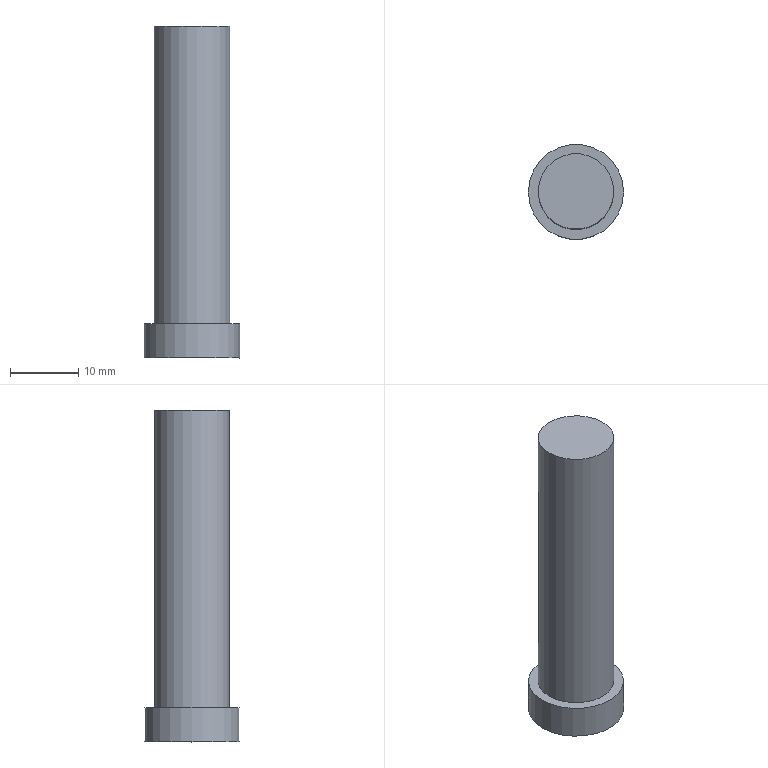Part | NX | features solid 2 | 1 solid | 5 faces | box 14 x 14 x 48.8 mm | volume 5008 mm3 | plane 3 | cylinder 2 | commonest cylinder face diameters 11.1 x1 14 x1
STEP:
#1=CARTESIAN_POINT('',(3033.266,-809.538,812.716));
#2=VERTEX_POINT('',#1);
#3=CARTESIAN_POINT('',(3040.266,-809.538,812.716));
#4=DIRECTION('',(0.,0.,1.));
#5=DIRECTION('',(-1.,0.,0.));
#6=AXIS2_PLACEMENT_3D('',#3,#4,#5);
#7=CIRCLE('',#6,7.);
#8=EDGE_CURVE('',#2,#2,#7,.T.);
#9=ORIENTED_EDGE('',*,*,#8,.F.);
#10=EDGE_LOOP('',(#9));
#11=FACE_BOUND('',#10,.T.);
#12=CARTESIAN_POINT('',(3040.266,-809.538,812.716));
#13=DIRECTION('',(0.,0.,-1.));
#14=DIRECTION('',(0.0349,-0.9994,0.));
#15=AXIS2_PLACEMENT_3D('',#12,#13,#14);
#16=PLANE('',#15);
#17=ADVANCED_FACE('',(#11),#16,.T.);
#18=CARTESIAN_POINT('',(3033.266,-809.538,817.716));
#19=VERTEX_POINT('',#18);
#20=CARTESIAN_POINT('',(3040.266,-809.538,817.716));
#21=DIRECTION('',(0.,0.,1.));
#22=DIRECTION('',(-1.,0.,0.));
#23=AXIS2_PLACEMENT_3D('',#20,#21,#22);
#24=CIRCLE('',#23,7.);
#25=EDGE_CURVE('',#19,#19,#24,.T.);
#26=ORIENTED_EDGE('',*,*,#25,.F.);
#27=EDGE_LOOP('',(#26));
#28=FACE_BOUND('',#27,.T.);
#29=ORIENTED_EDGE('',*,*,#8,.T.);
#30=EDGE_LOOP('',(#29));
#31=FACE_BOUND('',#30,.T.);
#32=CARTESIAN_POINT('',(3040.266,-809.538,855.716));
#33=DIRECTION('',(0.,0.,-1.));
#34=DIRECTION('',(0.,-1.,0.));
#35=AXIS2_PLACEMENT_3D('',#32,#33,#34);
#36=CYLINDRICAL_SURFACE('',#35,7.);
#37=ADVANCED_FACE('',(#28,#31),#36,.T.);
#38=CARTESIAN_POINT('',(3034.716,-809.538,817.716));
#39=VERTEX_POINT('',#38);
#40=CARTESIAN_POINT('',(3040.266,-809.538,817.716));
#41=DIRECTION('',(0.,0.,1.));
#42=DIRECTION('',(-1.,0.,0.));
#43=AXIS2_PLACEMENT_3D('',#40,#41,#42);
#44=CIRCLE('',#43,5.55);
#45=EDGE_CURVE('',#39,#39,#44,.F.);
#46=ORIENTED_EDGE('',*,*,#45,.T.);
#47=EDGE_LOOP('',(#46));
#48=FACE_BOUND('',#47,.T.);
#49=ORIENTED_EDGE('',*,*,#25,.T.);
#50=EDGE_LOOP('',(#49));
#51=FACE_BOUND('',#50,.T.);
#52=CARTESIAN_POINT('',(3040.266,-809.538,817.716));
#53=DIRECTION('',(0.,0.,-1.));
#54=DIRECTION('',(-1.,0.,0.));
#55=AXIS2_PLACEMENT_3D('',#52,#53,#54);
#56=PLANE('',#55);
#57=ADVANCED_FACE('',(#48,#51),#56,.F.);
#58=CARTESIAN_POINT('',(3045.816,-809.538,861.516));
#59=VERTEX_POINT('',#58);
#60=CARTESIAN_POINT('',(3040.266,-809.538,861.516));
#61=DIRECTION('',(0.,0.,-1.));
#62=DIRECTION('',(1.,0.,0.));
#63=AXIS2_PLACEMENT_3D('',#60,#61,#62);
#64=CIRCLE('',#63,5.55);
#65=EDGE_CURVE('',#59,#59,#64,.F.);
#66=ORIENTED_EDGE('',*,*,#65,.T.);
#67=EDGE_LOOP('',(#66));
#68=FACE_BOUND('',#67,.T.);
#69=CARTESIAN_POINT('',(3041.282,-809.207,861.516));
#70=DIRECTION('',(0.,0.,1.));
#71=DIRECTION('',(1.,0.,0.));
#72=AXIS2_PLACEMENT_3D('',#69,#70,#71);
#73=PLANE('',#72);
#74=ADVANCED_FACE('',(#68),#73,.T.);
#75=ORIENTED_EDGE('',*,*,#65,.F.);
#76=EDGE_LOOP('',(#75));
#77=FACE_BOUND('',#76,.T.);
#78=ORIENTED_EDGE('',*,*,#45,.F.);
#79=EDGE_LOOP('',(#78));
#80=FACE_BOUND('',#79,.T.);
#81=CARTESIAN_POINT('',(3040.266,-809.538,866.716));
#82=DIRECTION('',(0.,0.,-1.));
#83=DIRECTION('',(0.,-1.,0.));
#84=AXIS2_PLACEMENT_3D('',#81,#82,#83);
#85=CYLINDRICAL_SURFACE('',#84,5.55);
#86=ADVANCED_FACE('',(#77,#80),#85,.T.);
#87=CLOSED_SHELL('',(#17,#37,#57,#74,#86));
#88=MANIFOLD_SOLID_BREP('',#87);
#89=(LENGTH_UNIT()NAMED_UNIT(*)SI_UNIT(.MILLI.,.METRE.));
#90=UNCERTAINTY_MEASURE_WITH_UNIT(LENGTH_MEASURE(0.00001),#89,'','');
#91=(NAMED_UNIT(*)PLANE_ANGLE_UNIT()SI_UNIT($,.RADIAN.));
#92=(NAMED_UNIT(*)SI_UNIT($,.STERADIAN.)SOLID_ANGLE_UNIT());
#93=(GEOMETRIC_REPRESENTATION_CONTEXT(3)GLOBAL_UNCERTAINTY_ASSIGNED_CONTEXT((#90))GLOBAL_UNIT_ASSIGNED_CONTEXT((#89,#91,#92))REPRESENTATION_CONTEXT('',''));
#94=ADVANCED_BREP_SHAPE_REPRESENTATION('',(#88),#93);